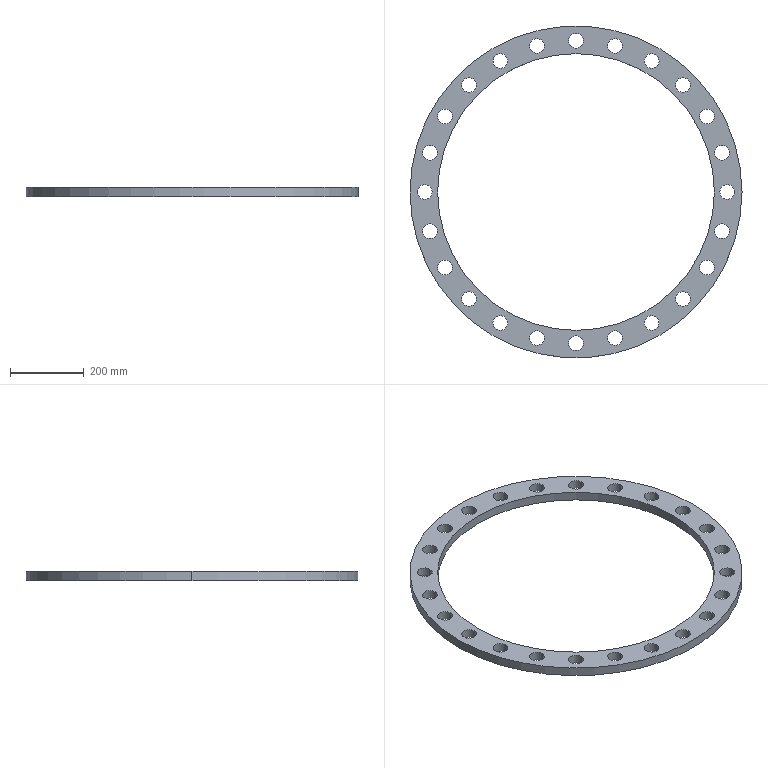Part | SolidWorks | features ICE 2, Extrusion 1 | 1 solid | 54 faces | box 900 x 900 x 25 mm | volume 4105669 mm3 | cylinder 52 | plane 2 | commonest cylinder face diameters 40 x48 750 x2 900 x2